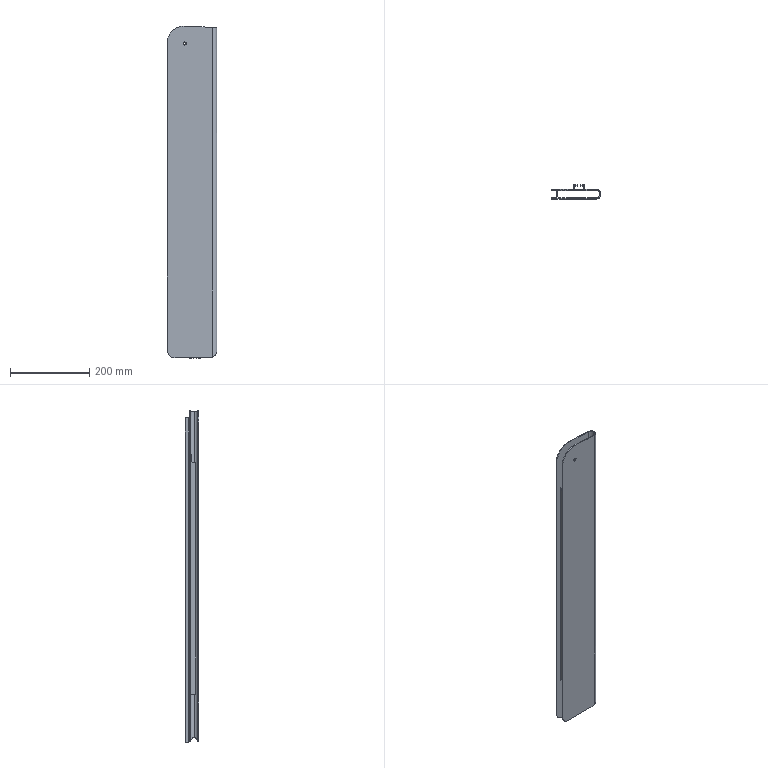Part | STEP file | 31E-01020TS12 | 1 solid | 83 faces | box 125 x 34 x 836 mm | volume 502303 mm3 | plane 42 | cylinder 41 | commonest cylinder face diameters 1 x8 2 x6 0.6 x4 4 x4 40 x3 6 x2